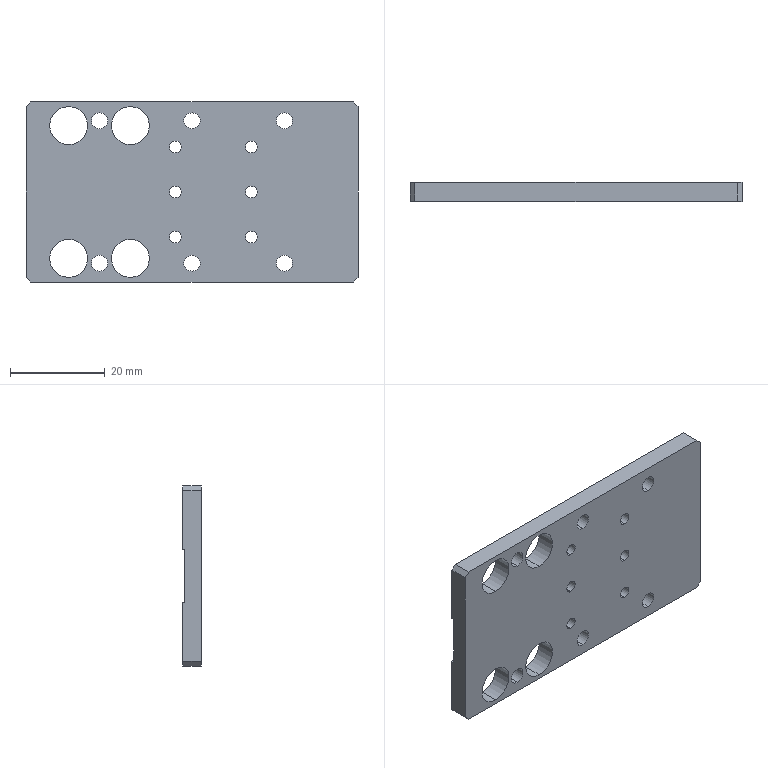Part | STEP file | Stopper bar cover plate | 1 solid | 46 faces | box 70 x 4 x 38 mm | volume 9112 mm3 | cylinder 32 | plane 14 | commonest cylinder face diameters 2.5 x12 3.4 x12 8 x8